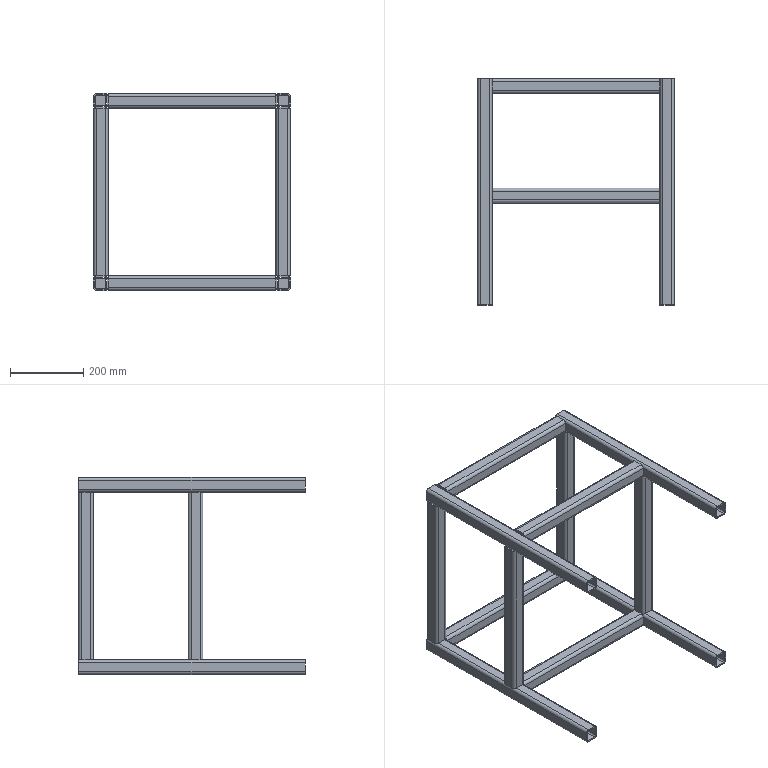Part | SolidWorks | features WeldCornerFeat 2, 3DProfileFeature 1, EndCap 1, WeldMemberFeat 1, WeldmentFeature 1 | 16 solids | 240 faces | box 540 x 620 x 540 mm | volume 3300618 mm3 | plane 144 | cylinder 96 | commonest cylinder face diameters 8 x48 16 x48